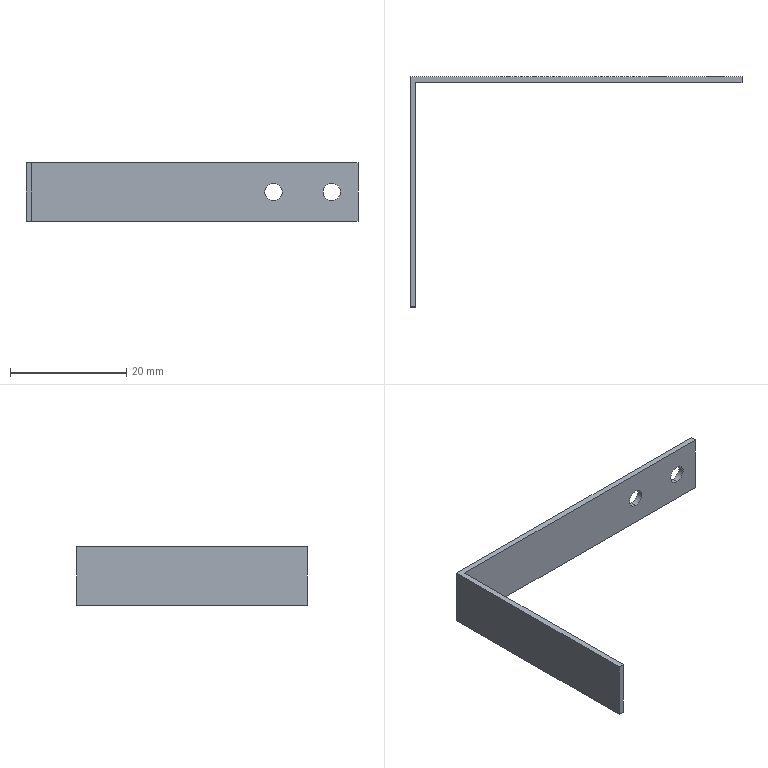Part | STEP file | 0230_206_Bracket | 1 solid | 12 faces | box 57 x 39.5 x 10 mm | volume 940.863 mm3 | plane 8 | cylinder 4 | commonest cylinder face diameters 3 x4
STEP:
#1=CARTESIAN_POINT('',(0.,0.,0.));
#2=DIRECTION('',(0.,0.,1.));
#3=DIRECTION('',(1.,0.,0.));
#4=AXIS2_PLACEMENT_3D('',#1,#2,#3);
#5=CARTESIAN_POINT('',(42.5,-1.,1.5));
#6=VERTEX_POINT('',#5);
#7=CARTESIAN_POINT('',(42.5,0.,1.5));
#8=VERTEX_POINT('',#7);
#9=CARTESIAN_POINT('',(42.5,0.,1.5));
#10=DIRECTION('',(0.,1.,0.));
#11=VECTOR('',#10,1.);
#12=LINE('',#9,#11);
#13=CARTESIAN_POINT('',(42.5,0.,0.));
#14=DIRECTION('',(0.,1.,0.));
#15=DIRECTION('',(0.,0.,1.));
#16=AXIS2_PLACEMENT_3D('',#13,#14,#15);
#17=CYLINDRICAL_SURFACE('',#16,1.5);
#18=CARTESIAN_POINT('',(6.283,0.));
#19=DIRECTION('',(0.,1.));
#20=VECTOR('',#19,1.);
#21=LINE('',#18,#20);
#22=(GEOMETRIC_REPRESENTATION_CONTEXT(2)PARAMETRIC_REPRESENTATION_CONTEXT()REPRESENTATION_CONTEXT('',''));
#23=DEFINITIONAL_REPRESENTATION('',(#21),#22);
#24=PCURVE('',#17,#23);
#25=CARTESIAN_POINT('',(42.5,0.,0.));
#26=DIRECTION('',(0.,1.,0.));
#27=DIRECTION('',(0.,0.,1.));
#28=AXIS2_PLACEMENT_3D('',#25,#26,#27);
#29=CYLINDRICAL_SURFACE('',#28,1.5);
#30=CARTESIAN_POINT('',(0.,0.));
#31=DIRECTION('',(0.,1.));
#32=VECTOR('',#31,1.);
#33=LINE('',#30,#32);
#34=(GEOMETRIC_REPRESENTATION_CONTEXT(2)PARAMETRIC_REPRESENTATION_CONTEXT()REPRESENTATION_CONTEXT('',''));
#35=DEFINITIONAL_REPRESENTATION('',(#33),#34);
#36=PCURVE('',#29,#35);
#37=SURFACE_CURVE('',#12,(#24,#36),.PCURVE_S1.);
#38=EDGE_CURVE('',#6,#8,#37,.T.);
#39=ORIENTED_EDGE('',*,*,#38,.T.);
#40=CARTESIAN_POINT('',(42.5,0.,-1.5));
#41=VERTEX_POINT('',#40);
#42=CARTESIAN_POINT('',(42.5,0.,0.));
#43=DIRECTION('',(0.,1.,0.));
#44=DIRECTION('',(0.,0.,1.));
#45=AXIS2_PLACEMENT_3D('',#42,#43,#44);
#46=CIRCLE('',#45,1.5);
#47=CARTESIAN_POINT('',(0.,0.));
#48=DIRECTION('',(1.,0.));
#49=VECTOR('',#48,1.);
#50=LINE('',#47,#49);
#51=(GEOMETRIC_REPRESENTATION_CONTEXT(2)PARAMETRIC_REPRESENTATION_CONTEXT()REPRESENTATION_CONTEXT('',''));
#52=DEFINITIONAL_REPRESENTATION('',(#50),#51);
#53=PCURVE('',#17,#52);
#54=CARTESIAN_POINT('',(57.,0.,-5.));
#55=DIRECTION('',(0.,1.,0.));
#56=DIRECTION('',(-1.,0.,0.));
#57=AXIS2_PLACEMENT_3D('',#54,#55,#56);
#58=PLANE('',#57);
#59=CARTESIAN_POINT('',(14.5,5.));
#60=DIRECTION('',(0.,1.));
#61=AXIS2_PLACEMENT_2D('',#59,#60);
#62=CIRCLE('',#61,1.5);
#63=(GEOMETRIC_REPRESENTATION_CONTEXT(2)PARAMETRIC_REPRESENTATION_CONTEXT()REPRESENTATION_CONTEXT('',''));
#64=DEFINITIONAL_REPRESENTATION('',(#62),#63);
#65=PCURVE('',#58,#64);
#66=SURFACE_CURVE('',#46,(#53,#65),.PCURVE_S1.);
#67=EDGE_CURVE('',#41,#8,#66,.T.);
#68=ORIENTED_EDGE('',*,*,#67,.F.);
#69=CARTESIAN_POINT('',(42.5,-1.,-1.5));
#70=VERTEX_POINT('',#69);
#71=CARTESIAN_POINT('',(42.5,0.,-1.5));
#72=DIRECTION('',(0.,1.,0.));
#73=VECTOR('',#72,1.);
#74=LINE('',#71,#73);
#75=CARTESIAN_POINT('',(3.142,0.));
#76=DIRECTION('',(0.,1.));
#77=VECTOR('',#76,1.);
#78=LINE('',#75,#77);
#79=(GEOMETRIC_REPRESENTATION_CONTEXT(2)PARAMETRIC_REPRESENTATION_CONTEXT()REPRESENTATION_CONTEXT('',''));
#80=DEFINITIONAL_REPRESENTATION('',(#78),#79);
#81=PCURVE('',#17,#80);
#82=CARTESIAN_POINT('',(3.142,0.));
#83=DIRECTION('',(0.,1.));
#84=VECTOR('',#83,1.);
#85=LINE('',#82,#84);
#86=(GEOMETRIC_REPRESENTATION_CONTEXT(2)PARAMETRIC_REPRESENTATION_CONTEXT()REPRESENTATION_CONTEXT('',''));
#87=DEFINITIONAL_REPRESENTATION('',(#85),#86);
#88=PCURVE('',#29,#87);
#89=SURFACE_CURVE('',#74,(#81,#88),.PCURVE_S1.);
#90=EDGE_CURVE('',#70,#41,#89,.T.);
#91=ORIENTED_EDGE('',*,*,#90,.F.);
#92=CARTESIAN_POINT('',(42.5,-1.,0.));
#93=DIRECTION('',(0.,1.,0.));
#94=DIRECTION('',(-1.,0.,0.));
#95=AXIS2_PLACEMENT_3D('',#92,#93,#94);
#96=CIRCLE('',#95,1.5);
#97=CARTESIAN_POINT('',(-1.571,-1.));
#98=DIRECTION('',(1.,0.));
#99=VECTOR('',#98,1.);
#100=LINE('',#97,#99);
#101=(GEOMETRIC_REPRESENTATION_CONTEXT(2)PARAMETRIC_REPRESENTATION_CONTEXT()REPRESENTATION_CONTEXT('',''));
#102=DEFINITIONAL_REPRESENTATION('',(#100),#101);
#103=PCURVE('',#17,#102);
#104=CARTESIAN_POINT('',(57.,-1.,-5.));
#105=DIRECTION('',(0.,1.,0.));
#106=DIRECTION('',(-1.,0.,0.));
#107=AXIS2_PLACEMENT_3D('',#104,#105,#106);
#108=PLANE('',#107);
#109=CARTESIAN_POINT('',(14.5,5.));
#110=DIRECTION('',(1.,0.));
#111=AXIS2_PLACEMENT_2D('',#109,#110);
#112=CIRCLE('',#111,1.5);
#113=(GEOMETRIC_REPRESENTATION_CONTEXT(2)PARAMETRIC_REPRESENTATION_CONTEXT()REPRESENTATION_CONTEXT('',''));
#114=DEFINITIONAL_REPRESENTATION('',(#112),#113);
#115=PCURVE('',#108,#114);
#116=SURFACE_CURVE('',#96,(#103,#115),.PCURVE_S1.);
#117=EDGE_CURVE('',#70,#6,#116,.T.);
#118=ORIENTED_EDGE('',*,*,#117,.T.);
#119=EDGE_LOOP('',(#39,#68,#91,#118));
#120=FACE_BOUND('',#119,.F.);
#121=ADVANCED_FACE('',(#120),#17,.F.);
#122=CARTESIAN_POINT('',(52.5,-1.,1.5));
#123=VERTEX_POINT('',#122);
#124=CARTESIAN_POINT('',(52.5,0.,1.5));
#125=VERTEX_POINT('',#124);
#126=CARTESIAN_POINT('',(52.5,0.,1.5));
#127=DIRECTION('',(0.,1.,0.));
#128=VECTOR('',#127,1.);
#129=LINE('',#126,#128);
#130=CARTESIAN_POINT('',(52.5,0.,0.));
#131=DIRECTION('',(0.,1.,0.));
#132=DIRECTION('',(0.,0.,1.));
#133=AXIS2_PLACEMENT_3D('',#130,#131,#132);
#134=CYLINDRICAL_SURFACE('',#133,1.5);
#135=CARTESIAN_POINT('',(6.283,0.));
#136=DIRECTION('',(0.,1.));
#137=VECTOR('',#136,1.);
#138=LINE('',#135,#137);
#139=(GEOMETRIC_REPRESENTATION_CONTEXT(2)PARAMETRIC_REPRESENTATION_CONTEXT()REPRESENTATION_CONTEXT('',''));
#140=DEFINITIONAL_REPRESENTATION('',(#138),#139);
#141=PCURVE('',#134,#140);
#142=CARTESIAN_POINT('',(52.5,0.,0.));
#143=DIRECTION('',(0.,1.,0.));
#144=DIRECTION('',(0.,0.,1.));
#145=AXIS2_PLACEMENT_3D('',#142,#143,#144);
#146=CYLINDRICAL_SURFACE('',#145,1.5);
#147=CARTESIAN_POINT('',(0.,0.));
#148=DIRECTION('',(0.,1.));
#149=VECTOR('',#148,1.);
#150=LINE('',#147,#149);
#151=(GEOMETRIC_REPRESENTATION_CONTEXT(2)PARAMETRIC_REPRESENTATION_CONTEXT()REPRESENTATION_CONTEXT('',''));
#152=DEFINITIONAL_REPRESENTATION('',(#150),#151);
#153=PCURVE('',#146,#152);
#154=SURFACE_CURVE('',#129,(#141,#153),.PCURVE_S1.);
#155=EDGE_CURVE('',#123,#125,#154,.T.);
#156=ORIENTED_EDGE('',*,*,#155,.T.);
#157=CARTESIAN_POINT('',(52.5,0.,-1.5));
#158=VERTEX_POINT('',#157);
#159=CARTESIAN_POINT('',(52.5,0.,0.));
#160=DIRECTION('',(0.,1.,0.));
#161=DIRECTION('',(0.,0.,1.));
#162=AXIS2_PLACEMENT_3D('',#159,#160,#161);
#163=CIRCLE('',#162,1.5);
#164=CARTESIAN_POINT('',(0.,0.));
#165=DIRECTION('',(1.,0.));
#166=VECTOR('',#165,1.);
#167=LINE('',#164,#166);
#168=(GEOMETRIC_REPRESENTATION_CONTEXT(2)PARAMETRIC_REPRESENTATION_CONTEXT()REPRESENTATION_CONTEXT('',''));
#169=DEFINITIONAL_REPRESENTATION('',(#167),#168);
#170=PCURVE('',#134,#169);
#171=CARTESIAN_POINT('',(4.5,5.));
#172=DIRECTION('',(0.,1.));
#173=AXIS2_PLACEMENT_2D('',#171,#172);
#174=CIRCLE('',#173,1.5);
#175=(GEOMETRIC_REPRESENTATION_CONTEXT(2)PARAMETRIC_REPRESENTATION_CONTEXT()REPRESENTATION_CONTEXT('',''));
#176=DEFINITIONAL_REPRESENTATION('',(#174),#175);
#177=PCURVE('',#58,#176);
#178=SURFACE_CURVE('',#163,(#170,#177),.PCURVE_S1.);
#179=EDGE_CURVE('',#158,#125,#178,.T.);
#180=ORIENTED_EDGE('',*,*,#179,.F.);
#181=CARTESIAN_POINT('',(52.5,-1.,-1.5));
#182=VERTEX_POINT('',#181);
#183=CARTESIAN_POINT('',(52.5,0.,-1.5));
#184=DIRECTION('',(0.,1.,0.));
#185=VECTOR('',#184,1.);
#186=LINE('',#183,#185);
#187=CARTESIAN_POINT('',(3.142,0.));
#188=DIRECTION('',(0.,1.));
#189=VECTOR('',#188,1.);
#190=LINE('',#187,#189);
#191=(GEOMETRIC_REPRESENTATION_CONTEXT(2)PARAMETRIC_REPRESENTATION_CONTEXT()REPRESENTATION_CONTEXT('',''));
#192=DEFINITIONAL_REPRESENTATION('',(#190),#191);
#193=PCURVE('',#134,#192);
#194=CARTESIAN_POINT('',(3.142,0.));
#195=DIRECTION('',(0.,1.));
#196=VECTOR('',#195,1.);
#197=LINE('',#194,#196);
#198=(GEOMETRIC_REPRESENTATION_CONTEXT(2)PARAMETRIC_REPRESENTATION_CONTEXT()REPRESENTATION_CONTEXT('',''));
#199=DEFINITIONAL_REPRESENTATION('',(#197),#198);
#200=PCURVE('',#146,#199);
#201=SURFACE_CURVE('',#186,(#193,#200),.PCURVE_S1.);
#202=EDGE_CURVE('',#182,#158,#201,.T.);
#203=ORIENTED_EDGE('',*,*,#202,.F.);
#204=CARTESIAN_POINT('',(52.5,-1.,0.));
#205=DIRECTION('',(0.,1.,0.));
#206=DIRECTION('',(-1.,0.,0.));
#207=AXIS2_PLACEMENT_3D('',#204,#205,#206);
#208=CIRCLE('',#207,1.5);
#209=CARTESIAN_POINT('',(-1.571,-1.));
#210=DIRECTION('',(1.,0.));
#211=VECTOR('',#210,1.);
#212=LINE('',#209,#211);
#213=(GEOMETRIC_REPRESENTATION_CONTEXT(2)PARAMETRIC_REPRESENTATION_CONTEXT()REPRESENTATION_CONTEXT('',''));
#214=DEFINITIONAL_REPRESENTATION('',(#212),#213);
#215=PCURVE('',#134,#214);
#216=CARTESIAN_POINT('',(4.5,5.));
#217=DIRECTION('',(1.,0.));
#218=AXIS2_PLACEMENT_2D('',#216,#217);
#219=CIRCLE('',#218,1.5);
#220=(GEOMETRIC_REPRESENTATION_CONTEXT(2)PARAMETRIC_REPRESENTATION_CONTEXT()REPRESENTATION_CONTEXT('',''));
#221=DEFINITIONAL_REPRESENTATION('',(#219),#220);
#222=PCURVE('',#108,#221);
#223=SURFACE_CURVE('',#208,(#215,#222),.PCURVE_S1.);
#224=EDGE_CURVE('',#182,#123,#223,.T.);
#225=ORIENTED_EDGE('',*,*,#224,.T.);
#226=EDGE_LOOP('',(#156,#180,#203,#225));
#227=FACE_BOUND('',#226,.F.);
#228=ADVANCED_FACE('',(#227),#134,.F.);
#229=CARTESIAN_POINT('',(0.,0.,5.));
#230=VERTEX_POINT('',#229);
#231=CARTESIAN_POINT('',(0.,-39.5,5.));
#232=VERTEX_POINT('',#231);
#233=CARTESIAN_POINT('',(0.,0.,5.));
#234=DIRECTION('',(0.,-1.,0.));
#235=VECTOR('',#234,1.);
#236=LINE('',#233,#235);
#237=CARTESIAN_POINT('',(0.,0.,-5.));
#238=DIRECTION('',(-1.,0.,0.));
#239=DIRECTION('',(0.,-1.,0.));
#240=AXIS2_PLACEMENT_3D('',#237,#238,#239);
#241=PLANE('',#240);
#242=CARTESIAN_POINT('',(0.,10.));
#243=DIRECTION('',(1.,0.));
#244=VECTOR('',#243,1.);
#245=LINE('',#242,#244);
#246=(GEOMETRIC_REPRESENTATION_CONTEXT(2)PARAMETRIC_REPRESENTATION_CONTEXT()REPRESENTATION_CONTEXT('',''));
#247=DEFINITIONAL_REPRESENTATION('',(#245),#246);
#248=PCURVE('',#241,#247);
#249=CARTESIAN_POINT('',(0.,-39.5,5.));
#250=DIRECTION('',(0.,0.,-1.));
#251=DIRECTION('',(-1.,0.,0.));
#252=AXIS2_PLACEMENT_3D('',#249,#250,#251);
#253=PLANE('',#252);
#254=CARTESIAN_POINT('',(0.,39.5));
#255=DIRECTION('',(0.,-1.));
#256=VECTOR('',#255,1.);
#257=LINE('',#254,#256);
#258=(GEOMETRIC_REPRESENTATION_CONTEXT(2)PARAMETRIC_REPRESENTATION_CONTEXT()REPRESENTATION_CONTEXT('',''));
#259=DEFINITIONAL_REPRESENTATION('',(#257),#258);
#260=PCURVE('',#253,#259);
#261=SURFACE_CURVE('',#236,(#248,#260),.PCURVE_S1.);
#262=EDGE_CURVE('',#230,#232,#261,.T.);
#263=ORIENTED_EDGE('',*,*,#262,.F.);
#264=CARTESIAN_POINT('',(0.,0.,-5.));
#265=VERTEX_POINT('',#264);
#266=CARTESIAN_POINT('',(0.,0.,-5.));
#267=DIRECTION('',(0.,0.,1.));
#268=VECTOR('',#267,1.);
#269=LINE('',#266,#268);
#270=CARTESIAN_POINT('',(0.,0.));
#271=DIRECTION('',(0.,1.));
#272=VECTOR('',#271,1.);
#273=LINE('',#270,#272);
#274=(GEOMETRIC_REPRESENTATION_CONTEXT(2)PARAMETRIC_REPRESENTATION_CONTEXT()REPRESENTATION_CONTEXT('',''));
#275=DEFINITIONAL_REPRESENTATION('',(#273),#274);
#276=PCURVE('',#241,#275);
#277=CARTESIAN_POINT('',(57.,0.));
#278=DIRECTION('',(0.,1.));
#279=VECTOR('',#278,1.);
#280=LINE('',#277,#279);
#281=(GEOMETRIC_REPRESENTATION_CONTEXT(2)PARAMETRIC_REPRESENTATION_CONTEXT()REPRESENTATION_CONTEXT('',''));
#282=DEFINITIONAL_REPRESENTATION('',(#280),#281);
#283=PCURVE('',#58,#282);
#284=SURFACE_CURVE('',#269,(#276,#283),.PCURVE_S1.);
#285=EDGE_CURVE('',#265,#230,#284,.T.);
#286=ORIENTED_EDGE('',*,*,#285,.F.);
#287=CARTESIAN_POINT('',(0.,-39.5,-5.));
#288=VERTEX_POINT('',#287);
#289=CARTESIAN_POINT('',(0.,0.,-5.));
#290=DIRECTION('',(0.,-1.,0.));
#291=VECTOR('',#290,1.);
#292=LINE('',#289,#291);
#293=CARTESIAN_POINT('',(0.,0.));
#294=DIRECTION('',(1.,0.));
#295=VECTOR('',#294,1.);
#296=LINE('',#293,#295);
#297=(GEOMETRIC_REPRESENTATION_CONTEXT(2)PARAMETRIC_REPRESENTATION_CONTEXT()REPRESENTATION_CONTEXT('',''));
#298=DEFINITIONAL_REPRESENTATION('',(#296),#297);
#299=PCURVE('',#241,#298);
#300=CARTESIAN_POINT('',(0.,-39.5,-5.));
#301=DIRECTION('',(0.,0.,-1.));
#302=DIRECTION('',(-1.,0.,0.));
#303=AXIS2_PLACEMENT_3D('',#300,#301,#302);
#304=PLANE('',#303);
#305=CARTESIAN_POINT('',(0.,39.5));
#306=DIRECTION('',(0.,-1.));
#307=VECTOR('',#306,1.);
#308=LINE('',#305,#307);
#309=(GEOMETRIC_REPRESENTATION_CONTEXT(2)PARAMETRIC_REPRESENTATION_CONTEXT()REPRESENTATION_CONTEXT('',''));
#310=DEFINITIONAL_REPRESENTATION('',(#308),#309);
#311=PCURVE('',#304,#310);
#312=SURFACE_CURVE('',#292,(#299,#311),.PCURVE_S1.);
#313=EDGE_CURVE('',#265,#288,#312,.T.);
#314=ORIENTED_EDGE('',*,*,#313,.T.);
#315=CARTESIAN_POINT('',(0.,-39.5,-5.));
#316=DIRECTION('',(0.,0.,1.));
#317=VECTOR('',#316,1.);
#318=LINE('',#315,#317);
#319=CARTESIAN_POINT('',(39.5,0.));
#320=DIRECTION('',(0.,1.));
#321=VECTOR('',#320,1.);
#322=LINE('',#319,#321);
#323=(GEOMETRIC_REPRESENTATION_CONTEXT(2)PARAMETRIC_REPRESENTATION_CONTEXT()REPRESENTATION_CONTEXT('',''));
#324=DEFINITIONAL_REPRESENTATION('',(#322),#323);
#325=PCURVE('',#241,#324);
#326=CARTESIAN_POINT('',(1.,-39.5,-5.));
#327=DIRECTION('',(0.,1.,0.));
#328=DIRECTION('',(0.,0.,1.));
#329=AXIS2_PLACEMENT_3D('',#326,#327,#328);
#330=PLANE('',#329);
#331=CARTESIAN_POINT('',(0.,-1.));
#332=DIRECTION('',(1.,0.));
#333=VECTOR('',#332,1.);
#334=LINE('',#331,#333);
#335=(GEOMETRIC_REPRESENTATION_CONTEXT(2)PARAMETRIC_REPRESENTATION_CONTEXT()REPRESENTATION_CONTEXT('',''));
#336=DEFINITIONAL_REPRESENTATION('',(#334),#335);
#337=PCURVE('',#330,#336);
#338=SURFACE_CURVE('',#318,(#325,#337),.PCURVE_S1.);
#339=EDGE_CURVE('',#288,#232,#338,.T.);
#340=ORIENTED_EDGE('',*,*,#339,.T.);
#341=EDGE_LOOP('',(#263,#286,#314,#340));
#342=FACE_BOUND('',#341,.T.);
#343=ADVANCED_FACE('',(#342),#241,.T.);
#344=CARTESIAN_POINT('',(42.5,0.,0.));
#345=DIRECTION('',(0.,1.,0.));
#346=DIRECTION('',(0.,0.,1.));
#347=AXIS2_PLACEMENT_3D('',#344,#345,#346);
#348=CIRCLE('',#347,1.5);
#349=CARTESIAN_POINT('',(14.5,5.));
#350=DIRECTION('',(0.,1.));
#351=AXIS2_PLACEMENT_2D('',#349,#350);
#352=CIRCLE('',#351,1.5);
#353=(GEOMETRIC_REPRESENTATION_CONTEXT(2)PARAMETRIC_REPRESENTATION_CONTEXT()REPRESENTATION_CONTEXT('',''));
#354=DEFINITIONAL_REPRESENTATION('',(#352),#353);
#355=PCURVE('',#58,#354);
#356=CARTESIAN_POINT('',(0.,0.));
#357=DIRECTION('',(1.,0.));
#358=VECTOR('',#357,1.);
#359=LINE('',#356,#358);
#360=(GEOMETRIC_REPRESENTATION_CONTEXT(2)PARAMETRIC_REPRESENTATION_CONTEXT()REPRESENTATION_CONTEXT('',''));
#361=DEFINITIONAL_REPRESENTATION('',(#359),#360);
#362=PCURVE('',#29,#361);
#363=SURFACE_CURVE('',#348,(#355,#362),.PCURVE_S1.);
#364=EDGE_CURVE('',#8,#41,#363,.T.);
#365=ORIENTED_EDGE('',*,*,#364,.F.);
#366=ORIENTED_EDGE('',*,*,#67,.F.);
#367=EDGE_LOOP('',(#365,#366));
#368=FACE_BOUND('',#367,.T.);
#369=CARTESIAN_POINT('',(52.5,0.,0.));
#370=DIRECTION('',(0.,1.,0.));
#371=DIRECTION('',(0.,0.,1.));
#372=AXIS2_PLACEMENT_3D('',#369,#370,#371);
#373=CIRCLE('',#372,1.5);
#374=CARTESIAN_POINT('',(4.5,5.));
#375=DIRECTION('',(0.,1.));
#376=AXIS2_PLACEMENT_2D('',#374,#375);
#377=CIRCLE('',#376,1.5);
#378=(GEOMETRIC_REPRESENTATION_CONTEXT(2)PARAMETRIC_REPRESENTATION_CONTEXT()REPRESENTATION_CONTEXT('',''));
#379=DEFINITIONAL_REPRESENTATION('',(#377),#378);
#380=PCURVE('',#58,#379);
#381=CARTESIAN_POINT('',(0.,0.));
#382=DIRECTION('',(1.,0.));
#383=VECTOR('',#382,1.);
#384=LINE('',#381,#383);
#385=(GEOMETRIC_REPRESENTATION_CONTEXT(2)PARAMETRIC_REPRESENTATION_CONTEXT()REPRESENTATION_CONTEXT('',''));
#386=DEFINITIONAL_REPRESENTATION('',(#384),#385);
#387=PCURVE('',#146,#386);
#388=SURFACE_CURVE('',#373,(#380,#387),.PCURVE_S1.);
#389=EDGE_CURVE('',#125,#158,#388,.T.);
#390=ORIENTED_EDGE('',*,*,#389,.F.);
#391=ORIENTED_EDGE('',*,*,#179,.F.);
#392=EDGE_LOOP('',(#390,#391));
#393=FACE_BOUND('',#392,.T.);
#394=CARTESIAN_POINT('',(57.,0.,5.));
#395=VERTEX_POINT('',#394);
#396=CARTESIAN_POINT('',(57.,0.,5.));
#397=DIRECTION('',(-1.,0.,0.));
#398=VECTOR('',#397,1.);
#399=LINE('',#396,#398);
#400=CARTESIAN_POINT('',(0.,10.));
#401=DIRECTION('',(1.,0.));
#402=VECTOR('',#401,1.);
#403=LINE('',#400,#402);
#404=(GEOMETRIC_REPRESENTATION_CONTEXT(2)PARAMETRIC_REPRESENTATION_CONTEXT()REPRESENTATION_CONTEXT('',''));
#405=DEFINITIONAL_REPRESENTATION('',(#403),#404);
#406=PCURVE('',#58,#405);
#407=CARTESIAN_POINT('',(-57.,39.5));
#408=DIRECTION('',(1.,0.));
#409=VECTOR('',#408,1.);
#410=LINE('',#407,#409);
#411=(GEOMETRIC_REPRESENTATION_CONTEXT(2)PARAMETRIC_REPRESENTATION_CONTEXT()REPRESENTATION_CONTEXT('',''));
#412=DEFINITIONAL_REPRESENTATION('',(#410),#411);
#413=PCURVE('',#253,#412);
#414=SURFACE_CURVE('',#399,(#406,#413),.PCURVE_S1.);
#415=EDGE_CURVE('',#395,#230,#414,.T.);
#416=ORIENTED_EDGE('',*,*,#415,.F.);
#417=CARTESIAN_POINT('',(57.,0.,-5.));
#418=VERTEX_POINT('',#417);
#419=CARTESIAN_POINT('',(57.,0.,-5.));
#420=DIRECTION('',(0.,0.,1.));
#421=VECTOR('',#420,1.);
#422=LINE('',#419,#421);
#423=CARTESIAN_POINT('',(0.,0.));
#424=DIRECTION('',(0.,1.));
#425=VECTOR('',#424,1.);
#426=LINE('',#423,#425);
#427=(GEOMETRIC_REPRESENTATION_CONTEXT(2)PARAMETRIC_REPRESENTATION_CONTEXT()REPRESENTATION_CONTEXT('',''));
#428=DEFINITIONAL_REPRESENTATION('',(#426),#427);
#429=PCURVE('',#58,#428);
#430=CARTESIAN_POINT('',(57.,0.,-5.));
#431=DIRECTION('',(-1.,0.,0.));
#432=DIRECTION('',(0.,0.,1.));
#433=AXIS2_PLACEMENT_3D('',#430,#431,#432);
#434=PLANE('',#433);
#435=CARTESIAN_POINT('',(0.,0.));
#436=DIRECTION('',(1.,0.));
#437=VECTOR('',#436,1.);
#438=LINE('',#435,#437);
#439=(GEOMETRIC_REPRESENTATION_CONTEXT(2)PARAMETRIC_REPRESENTATION_CONTEXT()REPRESENTATION_CONTEXT('',''));
#440=DEFINITIONAL_REPRESENTATION('',(#438),#439);
#441=PCURVE('',#434,#440);
#442=SURFACE_CURVE('',#422,(#429,#441),.PCURVE_S1.);
#443=EDGE_CURVE('',#418,#395,#442,.T.);
#444=ORIENTED_EDGE('',*,*,#443,.F.);
#445=CARTESIAN_POINT('',(57.,0.,-5.));
#446=DIRECTION('',(-1.,0.,0.));
#447=VECTOR('',#446,1.);
#448=LINE('',#445,#447);
#449=CARTESIAN_POINT('',(0.,0.));
#450=DIRECTION('',(1.,0.));
#451=VECTOR('',#450,1.);
#452=LINE('',#449,#451);
#453=(GEOMETRIC_REPRESENTATION_CONTEXT(2)PARAMETRIC_REPRESENTATION_CONTEXT()REPRESENTATION_CONTEXT('',''));
#454=DEFINITIONAL_REPRESENTATION('',(#452),#453);
#455=PCURVE('',#58,#454);
#456=CARTESIAN_POINT('',(-57.,39.5));
#457=DIRECTION('',(1.,0.));
#458=VECTOR('',#457,1.);
#459=LINE('',#456,#458);
#460=(GEOMETRIC_REPRESENTATION_CONTEXT(2)PARAMETRIC_REPRESENTATION_CONTEXT()REPRESENTATION_CONTEXT('',''));
#461=DEFINITIONAL_REPRESENTATION('',(#459),#460);
#462=PCURVE('',#304,#461);
#463=SURFACE_CURVE('',#448,(#455,#462),.PCURVE_S1.);
#464=EDGE_CURVE('',#418,#265,#463,.T.);
#465=ORIENTED_EDGE('',*,*,#464,.T.);
#466=ORIENTED_EDGE('',*,*,#285,.T.);
#467=EDGE_LOOP('',(#416,#444,#465,#466));
#468=FACE_BOUND('',#467,.T.);
#469=ADVANCED_FACE('',(#368,#393,#468),#58,.T.);
#470=CARTESIAN_POINT('',(57.,-1.,5.));
#471=VERTEX_POINT('',#470);
#472=CARTESIAN_POINT('',(57.,0.,5.));
#473=DIRECTION('',(0.,-1.,0.));
#474=VECTOR('',#473,1.);
#475=LINE('',#472,#474);
#476=CARTESIAN_POINT('',(10.,0.));
#477=DIRECTION('',(0.,-1.));
#478=VECTOR('',#477,1.);
#479=LINE('',#476,#478);
#480=(GEOMETRIC_REPRESENTATION_CONTEXT(2)PARAMETRIC_REPRESENTATION_CONTEXT()REPRESENTATION_CONTEXT('',''));
#481=DEFINITIONAL_REPRESENTATION('',(#479),#480);
#482=PCURVE('',#434,#481);
#483=CARTESIAN_POINT('',(-57.,39.5));
#484=DIRECTION('',(0.,-1.));
#485=VECTOR('',#484,1.);
#486=LINE('',#483,#485);
#487=(GEOMETRIC_REPRESENTATION_CONTEXT(2)PARAMETRIC_REPRESENTATION_CONTEXT()REPRESENTATION_CONTEXT('',''));
#488=DEFINITIONAL_REPRESENTATION('',(#486),#487);
#489=PCURVE('',#253,#488);
#490=SURFACE_CURVE('',#475,(#482,#489),.PCURVE_S1.);
#491=EDGE_CURVE('',#395,#471,#490,.T.);
#492=ORIENTED_EDGE('',*,*,#491,.T.);
#493=CARTESIAN_POINT('',(57.,-1.,-5.));
#494=VERTEX_POINT('',#493);
#495=CARTESIAN_POINT('',(57.,-1.,-5.));
#496=DIRECTION('',(0.,0.,1.));
#497=VECTOR('',#496,1.);
#498=LINE('',#495,#497);
#499=CARTESIAN_POINT('',(0.,-1.));
#500=DIRECTION('',(1.,0.));
#501=VECTOR('',#500,1.);
#502=LINE('',#499,#501);
#503=(GEOMETRIC_REPRESENTATION_CONTEXT(2)PARAMETRIC_REPRESENTATION_CONTEXT()REPRESENTATION_CONTEXT('',''));
#504=DEFINITIONAL_REPRESENTATION('',(#502),#503);
#505=PCURVE('',#434,#504);
#506=CARTESIAN_POINT('',(0.,0.));
#507=DIRECTION('',(0.,1.));
#508=VECTOR('',#507,1.);
#509=LINE('',#506,#508);
#510=(GEOMETRIC_REPRESENTATION_CONTEXT(2)PARAMETRIC_REPRESENTATION_CONTEXT()REPRESENTATION_CONTEXT('',''));
#511=DEFINITIONAL_REPRESENTATION('',(#509),#510);
#512=PCURVE('',#108,#511);
#513=SURFACE_CURVE('',#498,(#505,#512),.PCURVE_S1.);
#514=EDGE_CURVE('',#494,#471,#513,.T.);
#515=ORIENTED_EDGE('',*,*,#514,.F.);
#516=CARTESIAN_POINT('',(57.,0.,-5.));
#517=DIRECTION('',(0.,-1.,0.));
#518=VECTOR('',#517,1.);
#519=LINE('',#516,#518);
#520=CARTESIAN_POINT('',(0.,0.));
#521=DIRECTION('',(0.,-1.));
#522=VECTOR('',#521,1.);
#523=LINE('',#520,#522);
#524=(GEOMETRIC_REPRESENTATION_CONTEXT(2)PARAMETRIC_REPRESENTATION_CONTEXT()REPRESENTATION_CONTEXT('',''));
#525=DEFINITIONAL_REPRESENTATION('',(#523),#524);
#526=PCURVE('',#434,#525);
#527=CARTESIAN_POINT('',(-57.,39.5));
#528=DIRECTION('',(0.,-1.));
#529=VECTOR('',#528,1.);
#530=LINE('',#527,#529);
#531=(GEOMETRIC_REPRESENTATION_CONTEXT(2)PARAMETRIC_REPRESENTATION_CONTEXT()REPRESENTATION_CONTEXT('',''));
#532=DEFINITIONAL_REPRESENTATION('',(#530),#531);
#533=PCURVE('',#304,#532);
#534=SURFACE_CURVE('',#519,(#526,#533),.PCURVE_S1.);
#535=EDGE_CURVE('',#418,#494,#534,.T.);
#536=ORIENTED_EDGE('',*,*,#535,.F.);
#537=ORIENTED_EDGE('',*,*,#443,.T.);
#538=EDGE_LOOP('',(#492,#515,#536,#537));
#539=FACE_BOUND('',#538,.T.);
#540=ADVANCED_FACE('',(#539),#434,.F.);
#541=CARTESIAN_POINT('',(42.5,-1.,0.));
#542=DIRECTION('',(0.,1.,0.));
#543=DIRECTION('',(-1.,0.,0.));
#544=AXIS2_PLACEMENT_3D('',#541,#542,#543);
#545=CIRCLE('',#544,1.5);
#546=CARTESIAN_POINT('',(14.5,5.));
#547=DIRECTION('',(1.,0.));
#548=AXIS2_PLACEMENT_2D('',#546,#547);
#549=CIRCLE('',#548,1.5);
#550=(GEOMETRIC_REPRESENTATION_CONTEXT(2)PARAMETRIC_REPRESENTATION_CONTEXT()REPRESENTATION_CONTEXT('',''));
#551=DEFINITIONAL_REPRESENTATION('',(#549),#550);
#552=PCURVE('',#108,#551);
#553=CARTESIAN_POINT('',(-1.571,-1.));
#554=DIRECTION('',(1.,0.));
#555=VECTOR('',#554,1.);
#556=LINE('',#553,#555);
#557=(GEOMETRIC_REPRESENTATION_CONTEXT(2)PARAMETRIC_REPRESENTATION_CONTEXT()REPRESENTATION_CONTEXT('',''));
#558=DEFINITIONAL_REPRESENTATION('',(#556),#557);
#559=PCURVE('',#29,#558);
#560=SURFACE_CURVE('',#545,(#552,#559),.PCURVE_S1.);
#561=EDGE_CURVE('',#6,#70,#560,.T.);
#562=ORIENTED_EDGE('',*,*,#561,.T.);
#563=ORIENTED_EDGE('',*,*,#117,.T.);
#564=EDGE_LOOP('',(#562,#563));
#565=FACE_BOUND('',#564,.T.);
#566=CARTESIAN_POINT('',(52.5,-1.,0.));
#567=DIRECTION('',(0.,1.,0.));
#568=DIRECTION('',(-1.,0.,0.));
#569=AXIS2_PLACEMENT_3D('',#566,#567,#568);
#570=CIRCLE('',#569,1.5);
#571=CARTESIAN_POINT('',(4.5,5.));
#572=DIRECTION('',(1.,0.));
#573=AXIS2_PLACEMENT_2D('',#571,#572);
#574=CIRCLE('',#573,1.5);
#575=(GEOMETRIC_REPRESENTATION_CONTEXT(2)PARAMETRIC_REPRESENTATION_CONTEXT()REPRESENTATION_CONTEXT('',''));
#576=DEFINITIONAL_REPRESENTATION('',(#574),#575);
#577=PCURVE('',#108,#576);
#578=CARTESIAN_POINT('',(-1.571,-1.));
#579=DIRECTION('',(1.,0.));
#580=VECTOR('',#579,1.);
#581=LINE('',#578,#580);
#582=(GEOMETRIC_REPRESENTATION_CONTEXT(2)PARAMETRIC_REPRESENTATION_CONTEXT()REPRESENTATION_CONTEXT('',''));
#583=DEFINITIONAL_REPRESENTATION('',(#581),#582);
#584=PCURVE('',#146,#583);
#585=SURFACE_CURVE('',#570,(#577,#584),.PCURVE_S1.);
#586=EDGE_CURVE('',#123,#182,#585,.T.);
#587=ORIENTED_EDGE('',*,*,#586,.T.);
#588=ORIENTED_EDGE('',*,*,#224,.T.);
#589=EDGE_LOOP('',(#587,#588));
#590=FACE_BOUND('',#589,.T.);
#591=CARTESIAN_POINT('',(1.,-1.,5.));
#592=VERTEX_POINT('',#591);
#593=CARTESIAN_POINT('',(57.,-1.,5.));
#594=DIRECTION('',(-1.,0.,0.));
#595=VECTOR('',#594,1.);
#596=LINE('',#593,#595);
#597=CARTESIAN_POINT('',(0.,10.));
#598=DIRECTION('',(1.,0.));
#599=VECTOR('',#598,1.);
#600=LINE('',#597,#599);
#601=(GEOMETRIC_REPRESENTATION_CONTEXT(2)PARAMETRIC_REPRESENTATION_CONTEXT()REPRESENTATION_CONTEXT('',''));
#602=DEFINITIONAL_REPRESENTATION('',(#600),#601);
#603=PCURVE('',#108,#602);
#604=CARTESIAN_POINT('',(-57.,38.5));
#605=DIRECTION('',(1.,0.));
#606=VECTOR('',#605,1.);
#607=LINE('',#604,#606);
#608=(GEOMETRIC_REPRESENTATION_CONTEXT(2)PARAMETRIC_REPRESENTATION_CONTEXT()REPRESENTATION_CONTEXT('',''));
#609=DEFINITIONAL_REPRESENTATION('',(#607),#608);
#610=PCURVE('',#253,#609);
#611=SURFACE_CURVE('',#596,(#603,#610),.PCURVE_S1.);
#612=EDGE_CURVE('',#471,#592,#611,.T.);
#613=ORIENTED_EDGE('',*,*,#612,.T.);
#614=CARTESIAN_POINT('',(1.,-1.,-5.));
#615=VERTEX_POINT('',#614);
#616=CARTESIAN_POINT('',(1.,-1.,-5.));
#617=DIRECTION('',(0.,0.,1.));
#618=VECTOR('',#617,1.);
#619=LINE('',#616,#618);
#620=CARTESIAN_POINT('',(56.,0.));
#621=DIRECTION('',(0.,1.));
#622=VECTOR('',#621,1.);
#623=LINE('',#620,#622);
#624=(GEOMETRIC_REPRESENTATION_CONTEXT(2)PARAMETRIC_REPRESENTATION_CONTEXT()REPRESENTATION_CONTEXT('',''));
#625=DEFINITIONAL_REPRESENTATION('',(#623),#624);
#626=PCURVE('',#108,#625);
#627=CARTESIAN_POINT('',(1.,0.,-5.));
#628=DIRECTION('',(-1.,0.,0.));
#629=DIRECTION('',(0.,-1.,0.));
#630=AXIS2_PLACEMENT_3D('',#627,#628,#629);
#631=PLANE('',#630);
#632=CARTESIAN_POINT('',(1.,0.));
#633=DIRECTION('',(0.,1.));
#634=VECTOR('',#633,1.);
#635=LINE('',#632,#634);
#636=(GEOMETRIC_REPRESENTATION_CONTEXT(2)PARAMETRIC_REPRESENTATION_CONTEXT()REPRESENTATION_CONTEXT('',''));
#637=DEFINITIONAL_REPRESENTATION('',(#635),#636);
#638=PCURVE('',#631,#637);
#639=SURFACE_CURVE('',#619,(#626,#638),.PCURVE_S1.);
#640=EDGE_CURVE('',#615,#592,#639,.T.);
#641=ORIENTED_EDGE('',*,*,#640,.F.);
#642=CARTESIAN_POINT('',(57.,-1.,-5.));
#643=DIRECTION('',(-1.,0.,0.));
#644=VECTOR('',#643,1.);
#645=LINE('',#642,#644);
#646=CARTESIAN_POINT('',(0.,0.));
#647=DIRECTION('',(1.,0.));
#648=VECTOR('',#647,1.);
#649=LINE('',#646,#648);
#650=(GEOMETRIC_REPRESENTATION_CONTEXT(2)PARAMETRIC_REPRESENTATION_CONTEXT()REPRESENTATION_CONTEXT('',''));
#651=DEFINITIONAL_REPRESENTATION('',(#649),#650);
#652=PCURVE('',#108,#651);
#653=CARTESIAN_POINT('',(-57.,38.5));
#654=DIRECTION('',(1.,0.));
#655=VECTOR('',#654,1.);
#656=LINE('',#653,#655);
#657=(GEOMETRIC_REPRESENTATION_CONTEXT(2)PARAMETRIC_REPRESENTATION_CONTEXT()REPRESENTATION_CONTEXT('',''));
#658=DEFINITIONAL_REPRESENTATION('',(#656),#657);
#659=PCURVE('',#304,#658);
#660=SURFACE_CURVE('',#645,(#652,#659),.PCURVE_S1.);
#661=EDGE_CURVE('',#494,#615,#660,.T.);
#662=ORIENTED_EDGE('',*,*,#661,.F.);
#663=ORIENTED_EDGE('',*,*,#514,.T.);
#664=EDGE_LOOP('',(#613,#641,#662,#663));
#665=FACE_BOUND('',#664,.T.);
#666=ADVANCED_FACE('',(#565,#590,#665),#108,.F.);
#667=CARTESIAN_POINT('',(1.,-39.5,5.));
#668=VERTEX_POINT('',#667);
#669=CARTESIAN_POINT('',(1.,0.,5.));
#670=DIRECTION('',(0.,-1.,0.));
#671=VECTOR('',#670,1.);
#672=LINE('',#669,#671);
#673=CARTESIAN_POINT('',(0.,10.));
#674=DIRECTION('',(1.,0.));
#675=VECTOR('',#674,1.);
#676=LINE('',#673,#675);
#677=(GEOMETRIC_REPRESENTATION_CONTEXT(2)PARAMETRIC_REPRESENTATION_CONTEXT()REPRESENTATION_CONTEXT('',''));
#678=DEFINITIONAL_REPRESENTATION('',(#676),#677);
#679=PCURVE('',#631,#678);
#680=CARTESIAN_POINT('',(-1.,39.5));
#681=DIRECTION('',(0.,-1.));
#682=VECTOR('',#681,1.);
#683=LINE('',#680,#682);
#684=(GEOMETRIC_REPRESENTATION_CONTEXT(2)PARAMETRIC_REPRESENTATION_CONTEXT()REPRESENTATION_CONTEXT('',''));
#685=DEFINITIONAL_REPRESENTATION('',(#683),#684);
#686=PCURVE('',#253,#685);
#687=SURFACE_CURVE('',#672,(#679,#686),.PCURVE_S1.);
#688=EDGE_CURVE('',#592,#668,#687,.T.);
#689=ORIENTED_EDGE('',*,*,#688,.T.);
#690=CARTESIAN_POINT('',(1.,-39.5,-5.));
#691=VERTEX_POINT('',#690);
#692=CARTESIAN_POINT('',(1.,-39.5,-5.));
#693=DIRECTION('',(0.,0.,1.));
#694=VECTOR('',#693,1.);
#695=LINE('',#692,#694);
#696=CARTESIAN_POINT('',(39.5,0.));
#697=DIRECTION('',(0.,1.));
#698=VECTOR('',#697,1.);
#699=LINE('',#696,#698);
#700=(GEOMETRIC_REPRESENTATION_CONTEXT(2)PARAMETRIC_REPRESENTATION_CONTEXT()REPRESENTATION_CONTEXT('',''));
#701=DEFINITIONAL_REPRESENTATION('',(#699),#700);
#702=PCURVE('',#631,#701);
#703=CARTESIAN_POINT('',(0.,0.));
#704=DIRECTION('',(1.,0.));
#705=VECTOR('',#704,1.);
#706=LINE('',#703,#705);
#707=(GEOMETRIC_REPRESENTATION_CONTEXT(2)PARAMETRIC_REPRESENTATION_CONTEXT()REPRESENTATION_CONTEXT('',''));
#708=DEFINITIONAL_REPRESENTATION('',(#706),#707);
#709=PCURVE('',#330,#708);
#710=SURFACE_CURVE('',#695,(#702,#709),.PCURVE_S1.);
#711=EDGE_CURVE('',#691,#668,#710,.T.);
#712=ORIENTED_EDGE('',*,*,#711,.F.);
#713=CARTESIAN_POINT('',(1.,0.,-5.));
#714=DIRECTION('',(0.,-1.,0.));
#715=VECTOR('',#714,1.);
#716=LINE('',#713,#715);
#717=CARTESIAN_POINT('',(0.,0.));
#718=DIRECTION('',(1.,0.));
#719=VECTOR('',#718,1.);
#720=LINE('',#717,#719);
#721=(GEOMETRIC_REPRESENTATION_CONTEXT(2)PARAMETRIC_REPRESENTATION_CONTEXT()REPRESENTATION_CONTEXT('',''));
#722=DEFINITIONAL_REPRESENTATION('',(#720),#721);
#723=PCURVE('',#631,#722);
#724=CARTESIAN_POINT('',(-1.,39.5));
#725=DIRECTION('',(0.,-1.));
#726=VECTOR('',#725,1.);
#727=LINE('',#724,#726);
#728=(GEOMETRIC_REPRESENTATION_CONTEXT(2)PARAMETRIC_REPRESENTATION_CONTEXT()REPRESENTATION_CONTEXT('',''));
#729=DEFINITIONAL_REPRESENTATION('',(#727),#728);
#730=PCURVE('',#304,#729);
#731=SURFACE_CURVE('',#716,(#723,#730),.PCURVE_S1.);
#732=EDGE_CURVE('',#615,#691,#731,.T.);
#733=ORIENTED_EDGE('',*,*,#732,.F.);
#734=ORIENTED_EDGE('',*,*,#640,.T.);
#735=EDGE_LOOP('',(#689,#712,#733,#734));
#736=FACE_BOUND('',#735,.T.);
#737=ADVANCED_FACE('',(#736),#631,.F.);
#738=CARTESIAN_POINT('',(1.,-39.5,5.));
#739=DIRECTION('',(-1.,0.,0.));
#740=VECTOR('',#739,1.);
#741=LINE('',#738,#740);
#742=CARTESIAN_POINT('',(10.,0.));
#743=DIRECTION('',(0.,-1.));
#744=VECTOR('',#743,1.);
#745=LINE('',#742,#744);
#746=(GEOMETRIC_REPRESENTATION_CONTEXT(2)PARAMETRIC_REPRESENTATION_CONTEXT()REPRESENTATION_CONTEXT('',''));
#747=DEFINITIONAL_REPRESENTATION('',(#745),#746);
#748=PCURVE('',#330,#747);
#749=CARTESIAN_POINT('',(-1.,0.));
#750=DIRECTION('',(1.,0.));
#751=VECTOR('',#750,1.);
#752=LINE('',#749,#751);
#753=(GEOMETRIC_REPRESENTATION_CONTEXT(2)PARAMETRIC_REPRESENTATION_CONTEXT()REPRESENTATION_CONTEXT('',''));
#754=DEFINITIONAL_REPRESENTATION('',(#752),#753);
#755=PCURVE('',#253,#754);
#756=SURFACE_CURVE('',#741,(#748,#755),.PCURVE_S1.);
#757=EDGE_CURVE('',#668,#232,#756,.T.);
#758=ORIENTED_EDGE('',*,*,#757,.T.);
#759=ORIENTED_EDGE('',*,*,#339,.F.);
#760=CARTESIAN_POINT('',(1.,-39.5,-5.));
#761=DIRECTION('',(-1.,0.,0.));
#762=VECTOR('',#761,1.);
#763=LINE('',#760,#762);
#764=CARTESIAN_POINT('',(0.,0.));
#765=DIRECTION('',(0.,-1.));
#766=VECTOR('',#765,1.);
#767=LINE('',#764,#766);
#768=(GEOMETRIC_REPRESENTATION_CONTEXT(2)PARAMETRIC_REPRESENTATION_CONTEXT()REPRESENTATION_CONTEXT('',''));
#769=DEFINITIONAL_REPRESENTATION('',(#767),#768);
#770=PCURVE('',#330,#769);
#771=CARTESIAN_POINT('',(-1.,0.));
#772=DIRECTION('',(1.,0.));
#773=VECTOR('',#772,1.);
#774=LINE('',#771,#773);
#775=(GEOMETRIC_REPRESENTATION_CONTEXT(2)PARAMETRIC_REPRESENTATION_CONTEXT()REPRESENTATION_CONTEXT('',''));
#776=DEFINITIONAL_REPRESENTATION('',(#774),#775);
#777=PCURVE('',#304,#776);
#778=SURFACE_CURVE('',#763,(#770,#777),.PCURVE_S1.);
#779=EDGE_CURVE('',#691,#288,#778,.T.);
#780=ORIENTED_EDGE('',*,*,#779,.F.);
#781=ORIENTED_EDGE('',*,*,#711,.T.);
#782=EDGE_LOOP('',(#758,#759,#780,#781));
#783=FACE_BOUND('',#782,.T.);
#784=ADVANCED_FACE('',(#783),#330,.F.);
#785=ORIENTED_EDGE('',*,*,#313,.F.);
#786=ORIENTED_EDGE('',*,*,#464,.F.);
#787=ORIENTED_EDGE('',*,*,#535,.T.);
#788=ORIENTED_EDGE('',*,*,#661,.T.);
#789=ORIENTED_EDGE('',*,*,#732,.T.);
#790=ORIENTED_EDGE('',*,*,#779,.T.);
#791=EDGE_LOOP('',(#785,#786,#787,#788,#789,#790));
#792=FACE_BOUND('',#791,.T.);
#793=ADVANCED_FACE('',(#792),#304,.T.);
#794=ORIENTED_EDGE('',*,*,#262,.T.);
#795=ORIENTED_EDGE('',*,*,#757,.F.);
#796=ORIENTED_EDGE('',*,*,#688,.F.);
#797=ORIENTED_EDGE('',*,*,#612,.F.);
#798=ORIENTED_EDGE('',*,*,#491,.F.);
#799=ORIENTED_EDGE('',*,*,#415,.T.);
#800=EDGE_LOOP('',(#794,#795,#796,#797,#798,#799));
#801=FACE_BOUND('',#800,.T.);
#802=ADVANCED_FACE('',(#801),#253,.F.);
#803=ORIENTED_EDGE('',*,*,#389,.F.);
#804=ORIENTED_EDGE('',*,*,#155,.F.);
#805=ORIENTED_EDGE('',*,*,#586,.T.);
#806=ORIENTED_EDGE('',*,*,#202,.T.);
#807=EDGE_LOOP('',(#803,#804,#805,#806));
#808=FACE_BOUND('',#807,.F.);
#809=ADVANCED_FACE('',(#808),#146,.F.);
#810=ORIENTED_EDGE('',*,*,#364,.F.);
#811=ORIENTED_EDGE('',*,*,#38,.F.);
#812=ORIENTED_EDGE('',*,*,#561,.T.);
#813=ORIENTED_EDGE('',*,*,#90,.T.);
#814=EDGE_LOOP('',(#810,#811,#812,#813));
#815=FACE_BOUND('',#814,.F.);
#816=ADVANCED_FACE('',(#815),#29,.F.);
#817=CLOSED_SHELL('',(#121,#228,#343,#469,#540,#666,#737,#784,#793,#802,#809,#816));
#818=MANIFOLD_SOLID_BREP('',#817);
#819=(LENGTH_UNIT()NAMED_UNIT(*)SI_UNIT(.MILLI.,.METRE.));
#820=UNCERTAINTY_MEASURE_WITH_UNIT(LENGTH_MEASURE(0.0000001),#819,'','');
#821=(NAMED_UNIT(*)PLANE_ANGLE_UNIT()SI_UNIT($,.RADIAN.));
#822=(NAMED_UNIT(*)SI_UNIT($,.STERADIAN.)SOLID_ANGLE_UNIT());
#823=(GEOMETRIC_REPRESENTATION_CONTEXT(3)GLOBAL_UNCERTAINTY_ASSIGNED_CONTEXT((#820))GLOBAL_UNIT_ASSIGNED_CONTEXT((#819,#821,#822))REPRESENTATION_CONTEXT('',''));
#824=ADVANCED_BREP_SHAPE_REPRESENTATION('',(#4,#818),#823);